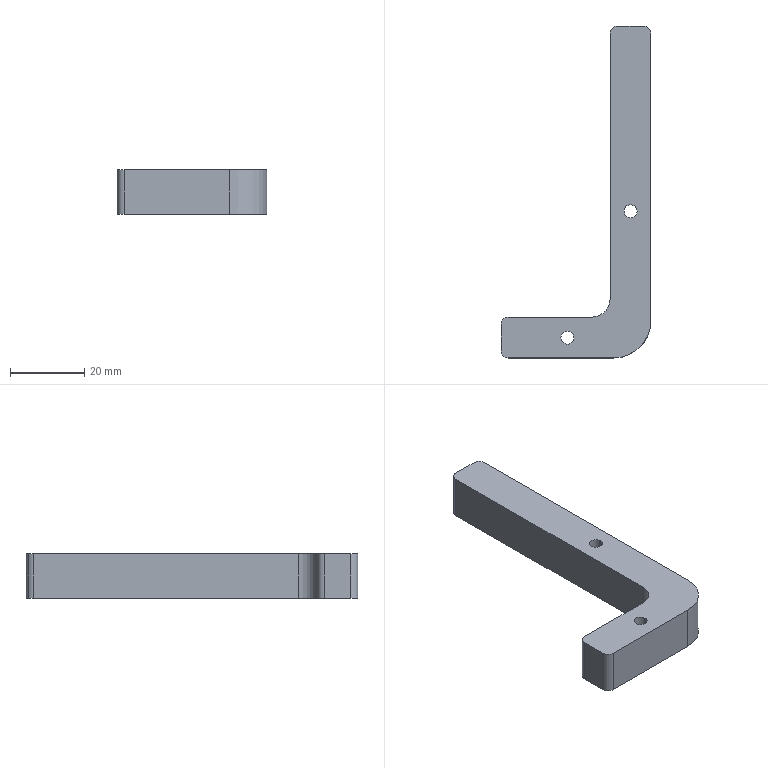Part | STEP file | ASND-0110-PWP TOP tu pang 20130814.sldasm-Part-5aq | 1 solid | 26 faces | box 40.426 x 89.575 x 12 mm | volume 15056 mm3 | cylinder 16 | plane 10 | commonest cylinder face diameters 4 x6 3.5 x4 6 x4 10 x1 20 x1